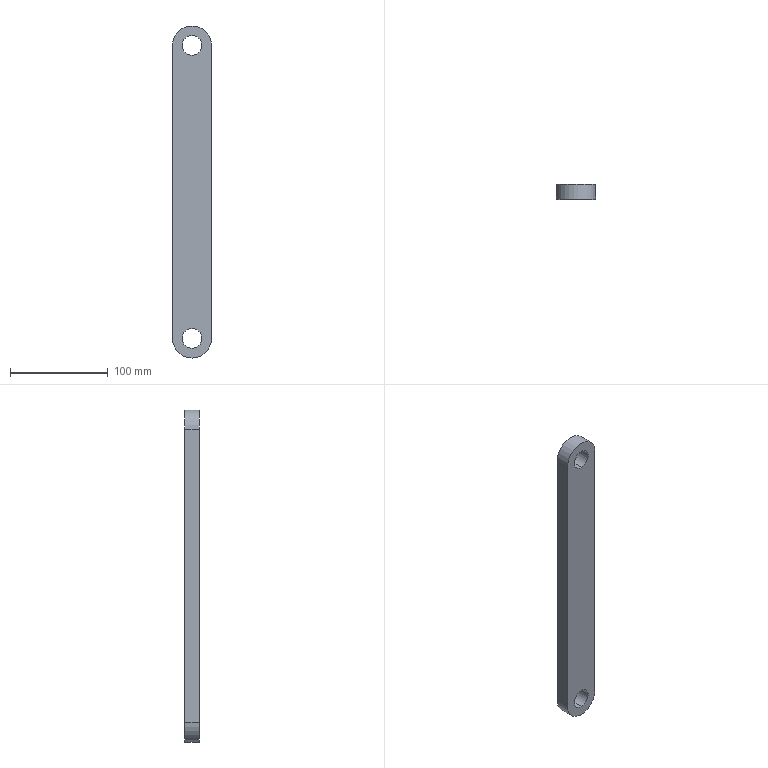Part | SolidWorks | features Extrusion 1 | 1 solid | 11 faces | box 40 x 15 x 340 mm | volume 189425 mm3 | cylinder 7 | plane 4 | commonest cylinder face diameters 20 x4 40 x3
STEP:
#1=CARTESIAN_POINT('',(0.,15.,-10.));
#2=VERTEX_POINT('',#1);
#3=CARTESIAN_POINT('',(0.,15.,10.));
#4=VERTEX_POINT('',#3);
#5=CARTESIAN_POINT('',(0.,15.,0.));
#6=DIRECTION('',(0.,1.,0.));
#7=DIRECTION('',(0.,0.,1.));
#8=AXIS2_PLACEMENT_3D('',#5,#6,#7);
#9=CIRCLE('',#8,10.);
#10=EDGE_CURVE('',#2,#4,#9,.T.);
#11=ORIENTED_EDGE('',*,*,#10,.T.);
#12=CARTESIAN_POINT('',(0.,0.,10.));
#13=VERTEX_POINT('',#12);
#14=CARTESIAN_POINT('',(0.,15.,10.));
#15=DIRECTION('',(0.,-1.,0.));
#16=VECTOR('',#15,1000.);
#17=LINE('',#14,#16);
#18=EDGE_CURVE('',#4,#13,#17,.T.);
#19=ORIENTED_EDGE('',*,*,#18,.T.);
#20=CARTESIAN_POINT('',(0.,0.,-10.));
#21=VERTEX_POINT('',#20);
#22=CARTESIAN_POINT('',(0.,0.,0.));
#23=DIRECTION('',(0.,1.,0.));
#24=DIRECTION('',(0.,0.,1.));
#25=AXIS2_PLACEMENT_3D('',#22,#23,#24);
#26=CIRCLE('',#25,10.);
#27=EDGE_CURVE('',#21,#13,#26,.T.);
#28=ORIENTED_EDGE('',*,*,#27,.F.);
#29=CARTESIAN_POINT('',(0.,15.,-10.));
#30=DIRECTION('',(0.,-1.,0.));
#31=VECTOR('',#30,1000.);
#32=LINE('',#29,#31);
#33=EDGE_CURVE('',#2,#21,#32,.T.);
#34=ORIENTED_EDGE('',*,*,#33,.F.);
#35=EDGE_LOOP('',(#11,#19,#28,#34));
#36=FACE_OUTER_BOUND('',#35,.T.);
#37=CARTESIAN_POINT('',(0.,15.,0.));
#38=DIRECTION('',(0.,-1.,0.));
#39=DIRECTION('',(0.,0.,-1.));
#40=AXIS2_PLACEMENT_3D('',#37,#38,#39);
#41=CYLINDRICAL_SURFACE('',#40,10.);
#42=ADVANCED_FACE('',(#36),#41,.F.);
#43=CARTESIAN_POINT('',(0.,15.,-310.));
#44=VERTEX_POINT('',#43);
#45=CARTESIAN_POINT('',(0.,15.,-290.));
#46=VERTEX_POINT('',#45);
#47=CARTESIAN_POINT('',(0.,15.,-300.));
#48=DIRECTION('',(0.,1.,0.));
#49=DIRECTION('',(0.,0.,1.));
#50=AXIS2_PLACEMENT_3D('',#47,#48,#49);
#51=CIRCLE('',#50,10.);
#52=EDGE_CURVE('',#44,#46,#51,.T.);
#53=ORIENTED_EDGE('',*,*,#52,.T.);
#54=CARTESIAN_POINT('',(0.,0.,-290.));
#55=VERTEX_POINT('',#54);
#56=CARTESIAN_POINT('',(0.,15.,-290.));
#57=DIRECTION('',(0.,-1.,0.));
#58=VECTOR('',#57,1000.);
#59=LINE('',#56,#58);
#60=EDGE_CURVE('',#46,#55,#59,.T.);
#61=ORIENTED_EDGE('',*,*,#60,.T.);
#62=CARTESIAN_POINT('',(0.,0.,-310.));
#63=VERTEX_POINT('',#62);
#64=CARTESIAN_POINT('',(0.,0.,-300.));
#65=DIRECTION('',(0.,1.,0.));
#66=DIRECTION('',(0.,0.,1.));
#67=AXIS2_PLACEMENT_3D('',#64,#65,#66);
#68=CIRCLE('',#67,10.);
#69=EDGE_CURVE('',#63,#55,#68,.T.);
#70=ORIENTED_EDGE('',*,*,#69,.F.);
#71=CARTESIAN_POINT('',(0.,15.,-310.));
#72=DIRECTION('',(0.,-1.,0.));
#73=VECTOR('',#72,1000.);
#74=LINE('',#71,#73);
#75=EDGE_CURVE('',#44,#63,#74,.T.);
#76=ORIENTED_EDGE('',*,*,#75,.F.);
#77=EDGE_LOOP('',(#53,#61,#70,#76));
#78=FACE_OUTER_BOUND('',#77,.T.);
#79=CARTESIAN_POINT('',(0.,15.,-300.));
#80=DIRECTION('',(0.,-1.,0.));
#81=DIRECTION('',(0.,0.,-1.));
#82=AXIS2_PLACEMENT_3D('',#79,#80,#81);
#83=CYLINDRICAL_SURFACE('',#82,10.);
#84=ADVANCED_FACE('',(#78),#83,.F.);
#85=CARTESIAN_POINT('',(0.,15.,-320.));
#86=VERTEX_POINT('',#85);
#87=CARTESIAN_POINT('',(-20.,15.,-300.));
#88=VERTEX_POINT('',#87);
#89=CARTESIAN_POINT('',(0.,15.,-300.));
#90=DIRECTION('',(0.,1.,0.));
#91=DIRECTION('',(0.,0.,1.));
#92=AXIS2_PLACEMENT_3D('',#89,#90,#91);
#93=CIRCLE('',#92,20.);
#94=EDGE_CURVE('',#86,#88,#93,.T.);
#95=ORIENTED_EDGE('',*,*,#94,.F.);
#96=CARTESIAN_POINT('',(0.,0.,-320.));
#97=VERTEX_POINT('',#96);
#98=CARTESIAN_POINT('',(0.,15.,-320.));
#99=DIRECTION('',(0.,-1.,0.));
#100=VECTOR('',#99,1000.);
#101=LINE('',#98,#100);
#102=EDGE_CURVE('',#86,#97,#101,.T.);
#103=ORIENTED_EDGE('',*,*,#102,.T.);
#104=CARTESIAN_POINT('',(-20.,0.,-300.));
#105=VERTEX_POINT('',#104);
#106=CARTESIAN_POINT('',(0.,0.,-300.));
#107=DIRECTION('',(0.,1.,0.));
#108=DIRECTION('',(0.,0.,1.));
#109=AXIS2_PLACEMENT_3D('',#106,#107,#108);
#110=CIRCLE('',#109,20.);
#111=EDGE_CURVE('',#97,#105,#110,.T.);
#112=ORIENTED_EDGE('',*,*,#111,.T.);
#113=CARTESIAN_POINT('',(-20.,15.,-300.));
#114=DIRECTION('',(0.,-1.,0.));
#115=VECTOR('',#114,1000.);
#116=LINE('',#113,#115);
#117=EDGE_CURVE('',#88,#105,#116,.T.);
#118=ORIENTED_EDGE('',*,*,#117,.F.);
#119=EDGE_LOOP('',(#95,#103,#112,#118));
#120=FACE_OUTER_BOUND('',#119,.T.);
#121=CARTESIAN_POINT('',(0.,15.,-300.));
#122=DIRECTION('',(0.,-1.,0.));
#123=DIRECTION('',(0.,0.,-1.));
#124=AXIS2_PLACEMENT_3D('',#121,#122,#123);
#125=CYLINDRICAL_SURFACE('',#124,20.);
#126=ADVANCED_FACE('',(#120),#125,.T.);
#127=ORIENTED_EDGE('',*,*,#52,.F.);
#128=CARTESIAN_POINT('',(0.,15.,-300.));
#129=DIRECTION('',(0.,1.,0.));
#130=DIRECTION('',(0.,0.,1.));
#131=AXIS2_PLACEMENT_3D('',#128,#129,#130);
#132=CIRCLE('',#131,10.);
#133=EDGE_CURVE('',#46,#44,#132,.T.);
#134=ORIENTED_EDGE('',*,*,#133,.F.);
#135=EDGE_LOOP('',(#127,#134));
#136=FACE_BOUND('',#135,.T.);
#137=CARTESIAN_POINT('',(-20.,15.,0.));
#138=VERTEX_POINT('',#137);
#139=CARTESIAN_POINT('',(20.,15.,0.));
#140=VERTEX_POINT('',#139);
#141=CARTESIAN_POINT('',(0.,15.,0.));
#142=DIRECTION('',(0.,1.,0.));
#143=DIRECTION('',(0.,0.,1.));
#144=AXIS2_PLACEMENT_3D('',#141,#142,#143);
#145=CIRCLE('',#144,20.);
#146=EDGE_CURVE('',#138,#140,#145,.T.);
#147=ORIENTED_EDGE('',*,*,#146,.T.);
#148=CARTESIAN_POINT('',(20.,15.,-300.));
#149=VERTEX_POINT('',#148);
#150=CARTESIAN_POINT('',(20.,15.,0.));
#151=DIRECTION('',(0.,0.,-1.));
#152=VECTOR('',#151,1000.);
#153=LINE('',#150,#152);
#154=EDGE_CURVE('',#140,#149,#153,.T.);
#155=ORIENTED_EDGE('',*,*,#154,.T.);
#156=CARTESIAN_POINT('',(0.,15.,-300.));
#157=DIRECTION('',(0.,1.,0.));
#158=DIRECTION('',(0.,0.,1.));
#159=AXIS2_PLACEMENT_3D('',#156,#157,#158);
#160=CIRCLE('',#159,20.);
#161=EDGE_CURVE('',#149,#86,#160,.T.);
#162=ORIENTED_EDGE('',*,*,#161,.T.);
#163=ORIENTED_EDGE('',*,*,#94,.T.);
#164=CARTESIAN_POINT('',(-20.,15.,0.));
#165=DIRECTION('',(0.,0.,1.));
#166=VECTOR('',#165,1000.);
#167=LINE('',#164,#166);
#168=EDGE_CURVE('',#88,#138,#167,.T.);
#169=ORIENTED_EDGE('',*,*,#168,.T.);
#170=EDGE_LOOP('',(#147,#155,#162,#163,#169));
#171=FACE_OUTER_BOUND('',#170,.T.);
#172=ORIENTED_EDGE('',*,*,#10,.F.);
#173=CARTESIAN_POINT('',(0.,15.,0.));
#174=DIRECTION('',(0.,1.,0.));
#175=DIRECTION('',(0.,0.,1.));
#176=AXIS2_PLACEMENT_3D('',#173,#174,#175);
#177=CIRCLE('',#176,10.);
#178=EDGE_CURVE('',#4,#2,#177,.T.);
#179=ORIENTED_EDGE('',*,*,#178,.F.);
#180=EDGE_LOOP('',(#172,#179));
#181=FACE_BOUND('',#180,.T.);
#182=CARTESIAN_POINT('',(0.,15.,0.));
#183=DIRECTION('',(0.,1.,0.));
#184=DIRECTION('',(0.,0.,1.));
#185=AXIS2_PLACEMENT_3D('',#182,#183,#184);
#186=PLANE('',#185);
#187=ADVANCED_FACE('',(#136,#171,#181),#186,.T.);
#188=CARTESIAN_POINT('',(-20.,0.,0.));
#189=VERTEX_POINT('',#188);
#190=CARTESIAN_POINT('',(20.,0.,0.));
#191=VERTEX_POINT('',#190);
#192=CARTESIAN_POINT('',(0.,0.,0.));
#193=DIRECTION('',(0.,1.,0.));
#194=DIRECTION('',(0.,0.,1.));
#195=AXIS2_PLACEMENT_3D('',#192,#193,#194);
#196=CIRCLE('',#195,20.);
#197=EDGE_CURVE('',#189,#191,#196,.T.);
#198=ORIENTED_EDGE('',*,*,#197,.F.);
#199=CARTESIAN_POINT('',(-20.,0.,0.));
#200=DIRECTION('',(0.,0.,1.));
#201=VECTOR('',#200,1000.);
#202=LINE('',#199,#201);
#203=EDGE_CURVE('',#105,#189,#202,.T.);
#204=ORIENTED_EDGE('',*,*,#203,.F.);
#205=ORIENTED_EDGE('',*,*,#111,.F.);
#206=CARTESIAN_POINT('',(20.,0.,-300.));
#207=VERTEX_POINT('',#206);
#208=CARTESIAN_POINT('',(0.,0.,-300.));
#209=DIRECTION('',(0.,1.,0.));
#210=DIRECTION('',(0.,0.,1.));
#211=AXIS2_PLACEMENT_3D('',#208,#209,#210);
#212=CIRCLE('',#211,20.);
#213=EDGE_CURVE('',#207,#97,#212,.T.);
#214=ORIENTED_EDGE('',*,*,#213,.F.);
#215=CARTESIAN_POINT('',(20.,0.,0.));
#216=DIRECTION('',(0.,0.,-1.));
#217=VECTOR('',#216,1000.);
#218=LINE('',#215,#217);
#219=EDGE_CURVE('',#191,#207,#218,.T.);
#220=ORIENTED_EDGE('',*,*,#219,.F.);
#221=EDGE_LOOP('',(#198,#204,#205,#214,#220));
#222=FACE_OUTER_BOUND('',#221,.T.);
#223=ORIENTED_EDGE('',*,*,#69,.T.);
#224=CARTESIAN_POINT('',(0.,0.,-300.));
#225=DIRECTION('',(0.,1.,0.));
#226=DIRECTION('',(0.,0.,1.));
#227=AXIS2_PLACEMENT_3D('',#224,#225,#226);
#228=CIRCLE('',#227,10.);
#229=EDGE_CURVE('',#55,#63,#228,.T.);
#230=ORIENTED_EDGE('',*,*,#229,.T.);
#231=EDGE_LOOP('',(#223,#230));
#232=FACE_BOUND('',#231,.T.);
#233=ORIENTED_EDGE('',*,*,#27,.T.);
#234=CARTESIAN_POINT('',(0.,0.,0.));
#235=DIRECTION('',(0.,1.,0.));
#236=DIRECTION('',(0.,0.,1.));
#237=AXIS2_PLACEMENT_3D('',#234,#235,#236);
#238=CIRCLE('',#237,10.);
#239=EDGE_CURVE('',#13,#21,#238,.T.);
#240=ORIENTED_EDGE('',*,*,#239,.T.);
#241=EDGE_LOOP('',(#233,#240));
#242=FACE_BOUND('',#241,.T.);
#243=CARTESIAN_POINT('',(0.,0.,0.));
#244=DIRECTION('',(0.,1.,0.));
#245=DIRECTION('',(0.,0.,1.));
#246=AXIS2_PLACEMENT_3D('',#243,#244,#245);
#247=PLANE('',#246);
#248=ADVANCED_FACE('',(#222,#232,#242),#247,.F.);
#249=ORIENTED_EDGE('',*,*,#197,.T.);
#250=CARTESIAN_POINT('',(20.,15.,0.));
#251=DIRECTION('',(0.,-1.,0.));
#252=VECTOR('',#251,1000.);
#253=LINE('',#250,#252);
#254=EDGE_CURVE('',#140,#191,#253,.T.);
#255=ORIENTED_EDGE('',*,*,#254,.F.);
#256=ORIENTED_EDGE('',*,*,#146,.F.);
#257=CARTESIAN_POINT('',(-20.,15.,0.));
#258=DIRECTION('',(0.,-1.,0.));
#259=VECTOR('',#258,1000.);
#260=LINE('',#257,#259);
#261=EDGE_CURVE('',#138,#189,#260,.T.);
#262=ORIENTED_EDGE('',*,*,#261,.T.);
#263=EDGE_LOOP('',(#249,#255,#256,#262));
#264=FACE_OUTER_BOUND('',#263,.T.);
#265=CARTESIAN_POINT('',(0.,15.,0.));
#266=DIRECTION('',(0.,-1.,0.));
#267=DIRECTION('',(0.,0.,-1.));
#268=AXIS2_PLACEMENT_3D('',#265,#266,#267);
#269=CYLINDRICAL_SURFACE('',#268,20.);
#270=ADVANCED_FACE('',(#264),#269,.T.);
#271=ORIENTED_EDGE('',*,*,#219,.T.);
#272=CARTESIAN_POINT('',(20.,15.,-300.));
#273=DIRECTION('',(0.,-1.,0.));
#274=VECTOR('',#273,1000.);
#275=LINE('',#272,#274);
#276=EDGE_CURVE('',#149,#207,#275,.T.);
#277=ORIENTED_EDGE('',*,*,#276,.F.);
#278=ORIENTED_EDGE('',*,*,#154,.F.);
#279=ORIENTED_EDGE('',*,*,#254,.T.);
#280=EDGE_LOOP('',(#271,#277,#278,#279));
#281=FACE_OUTER_BOUND('',#280,.T.);
#282=CARTESIAN_POINT('',(20.,15.,0.));
#283=DIRECTION('',(-1.,0.,0.));
#284=DIRECTION('',(0.,0.,1.));
#285=AXIS2_PLACEMENT_3D('',#282,#283,#284);
#286=PLANE('',#285);
#287=ADVANCED_FACE('',(#281),#286,.F.);
#288=ORIENTED_EDGE('',*,*,#102,.F.);
#289=ORIENTED_EDGE('',*,*,#161,.F.);
#290=ORIENTED_EDGE('',*,*,#276,.T.);
#291=ORIENTED_EDGE('',*,*,#213,.T.);
#292=EDGE_LOOP('',(#288,#289,#290,#291));
#293=FACE_OUTER_BOUND('',#292,.T.);
#294=CARTESIAN_POINT('',(0.,15.,-300.));
#295=DIRECTION('',(0.,-1.,0.));
#296=DIRECTION('',(0.,0.,-1.));
#297=AXIS2_PLACEMENT_3D('',#294,#295,#296);
#298=CYLINDRICAL_SURFACE('',#297,20.);
#299=ADVANCED_FACE('',(#293),#298,.T.);
#300=ORIENTED_EDGE('',*,*,#203,.T.);
#301=ORIENTED_EDGE('',*,*,#261,.F.);
#302=ORIENTED_EDGE('',*,*,#168,.F.);
#303=ORIENTED_EDGE('',*,*,#117,.T.);
#304=EDGE_LOOP('',(#300,#301,#302,#303));
#305=FACE_OUTER_BOUND('',#304,.T.);
#306=CARTESIAN_POINT('',(-20.,15.,0.));
#307=DIRECTION('',(1.,0.,0.));
#308=DIRECTION('',(0.,0.,-1.));
#309=AXIS2_PLACEMENT_3D('',#306,#307,#308);
#310=PLANE('',#309);
#311=ADVANCED_FACE('',(#305),#310,.F.);
#312=ORIENTED_EDGE('',*,*,#60,.F.);
#313=ORIENTED_EDGE('',*,*,#133,.T.);
#314=ORIENTED_EDGE('',*,*,#75,.T.);
#315=ORIENTED_EDGE('',*,*,#229,.F.);
#316=EDGE_LOOP('',(#312,#313,#314,#315));
#317=FACE_OUTER_BOUND('',#316,.T.);
#318=CARTESIAN_POINT('',(0.,15.,-300.));
#319=DIRECTION('',(0.,-1.,0.));
#320=DIRECTION('',(0.,0.,-1.));
#321=AXIS2_PLACEMENT_3D('',#318,#319,#320);
#322=CYLINDRICAL_SURFACE('',#321,10.);
#323=ADVANCED_FACE('',(#317),#322,.F.);
#324=ORIENTED_EDGE('',*,*,#18,.F.);
#325=ORIENTED_EDGE('',*,*,#178,.T.);
#326=ORIENTED_EDGE('',*,*,#33,.T.);
#327=ORIENTED_EDGE('',*,*,#239,.F.);
#328=EDGE_LOOP('',(#324,#325,#326,#327));
#329=FACE_OUTER_BOUND('',#328,.T.);
#330=CARTESIAN_POINT('',(0.,15.,0.));
#331=DIRECTION('',(0.,-1.,0.));
#332=DIRECTION('',(0.,0.,-1.));
#333=AXIS2_PLACEMENT_3D('',#330,#331,#332);
#334=CYLINDRICAL_SURFACE('',#333,10.);
#335=ADVANCED_FACE('',(#329),#334,.F.);
#336=CLOSED_SHELL('',(#42,#84,#126,#187,#248,#270,#287,#299,#311,#323,#335));
#337=MANIFOLD_SOLID_BREP('',#336);
#338=CARTESIAN_POINT('',(0.,0.,0.));
#339=DIRECTION('',(0.,0.,1.));
#340=DIRECTION('',(1.,0.,0.));
#341=AXIS2_PLACEMENT_3D('',#338,#339,#340);
#342=(LENGTH_UNIT()NAMED_UNIT(*)SI_UNIT(.MILLI.,.METRE.));
#343=UNCERTAINTY_MEASURE_WITH_UNIT(LENGTH_MEASURE(0.00001),#342,'','');
#344=(NAMED_UNIT(*)PLANE_ANGLE_UNIT()SI_UNIT($,.RADIAN.));
#345=(NAMED_UNIT(*)SI_UNIT($,.STERADIAN.)SOLID_ANGLE_UNIT());
#346=(GEOMETRIC_REPRESENTATION_CONTEXT(3)GLOBAL_UNCERTAINTY_ASSIGNED_CONTEXT((#343))GLOBAL_UNIT_ASSIGNED_CONTEXT((#342,#344,#345))REPRESENTATION_CONTEXT('',''));
#347=ADVANCED_BREP_SHAPE_REPRESENTATION('',(#337,#341),#346);